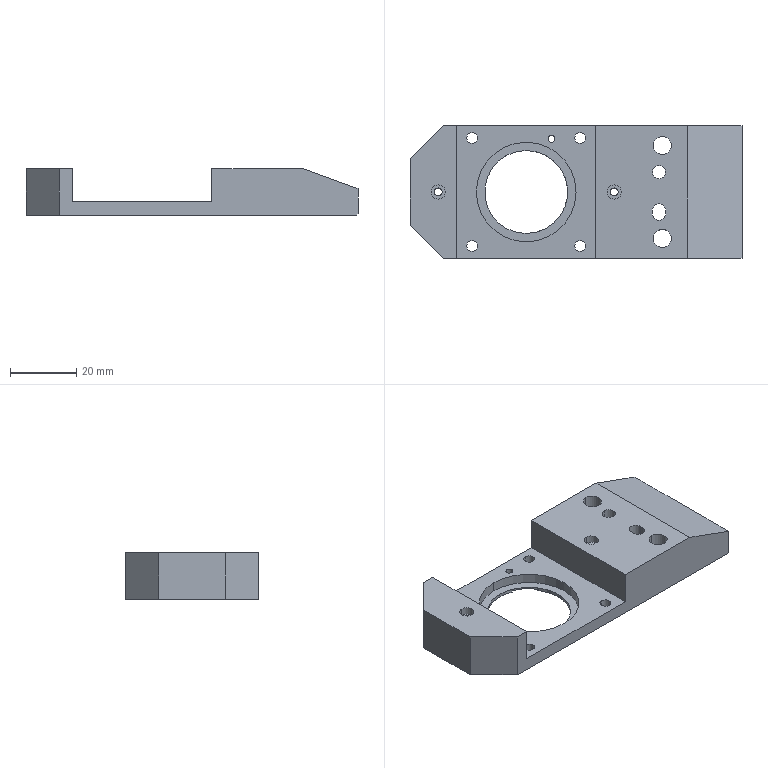NC program | NX | posted with a generic post | part box 100 x 40 x 14 mm
Lines 7056 to 8468 of 15435:
(DRILLING_COPY_1 , TOOL : ZXZ)
N14098 T20 M6
N14100 G54
N14102 G17 G0 G90 X-31.263 Y-16.263 S5000 M3
N14104 G43 Z30. H20
N14106 G94 G81 G98 Z-11. F250. R-7.
N14108 X-41.5 Y0. Z-1. R3.
N14110 X-31.263 Y16.263 Z-11. R-7.
N14112 X-7.4 Y16.
N14114 X1.263 Y16.263
N14116 X-15. Y0.
N14118 X1.263 Y-16.263
N14120 X11.5 Y0. Z-1. R3.
N14122 X26. Y14.
N14124 X25. Y6.
N14126 Y-5.5
N14128 X26. Y-14.
N14130 G80
N14132 G0 X26. Y-14. Z30.
N14134 M5
(DRILLING_COPY_1_COPY , TOOL : 3.3ZT)
N14136 T13 M6
N14138 G54
N14140 G17 G0 G90 X1.263 Y-16.263 S2000 M3
N14142 G43 Z30. H13
N14144 G94 G83 G98 Z-15.491 F150. Q2. R-7.
N14146 X-31.263
N14148 Y16.263
N14150 X1.263
N14152 G80
N14154 G0 X1.263 Y16.263 Z30.
N14156 M5
(TOOLCOMP11 , TOOL : D2.9XYD)
N14158 T11 M6
N14160 G54
N14162 G17 G0 G90 X-31.263 Y16.263 S4000 M3
N14164 G43 Z30. H11
N14166 Z-9.373
N14168 G42 G94 G1 X-31.19 Y16.195 F1000. D11
N14170 G2 X-31.327 Y15.983 Z-9.5 R0.134
N14172 X-31.327 Y15.983 Z-10.2 I0.064 J0.28
N14174 X-31.327 Y15.983 Z-10.9 I0.064 J0.28
N14176 X-31.327 Y15.983 Z-11.6 I0.064 J0.28
N14178 X-31.327 Y15.983 Z-12.3 I0.064 J0.28
N14180 X-31.327 Y15.983 Z-13. I0.064 J0.28
N14182 X-31.327 Y15.983 Z-13.7 I0.064 J0.28
N14184 X-31.327 Y16.544 Z-14. R0.287
N14186 X-31.19 Y16.332 Z-14.127 R0.134
N14188 G40
N14190 G1 X-31.263 Y16.263
N14192 G0 Z30.
N14194 Z-9.359
N14196 G42 G1 X-31.18 Y16.208
N14198 G2 X-31.347 Y15.898 Z-9.5 R0.183
N14200 X-31.347 Y15.898 Z-10.2 I0.083 J0.366
N14202 X-31.347 Y15.898 Z-10.9 I0.083 J0.366
N14204 X-31.347 Y15.898 Z-11.6 I0.083 J0.366
N14206 X-31.347 Y15.898 Z-12.3 I0.083 J0.366
N14208 X-31.347 Y15.898 Z-13. I0.083 J0.366
N14210 X-31.347 Y15.898 Z-13.7 I0.083 J0.366
N14212 X-31.347 Y16.629 Z-14. R0.375
N14214 X-31.18 Y16.319 Z-14.141 R0.183
N14216 G40
N14218 G1 X-31.263 Y16.263
N14220 G0 Z30.
N14222 Z-9.351
N14224 G42 G1 X-31.175 Y16.217
N14226 G2 X-31.366 Y15.813 Z-9.5 R0.229
N14228 X-31.366 Y15.813 Z-10.2 I0.103 J0.451
N14230 X-31.366 Y15.813 Z-10.9 I0.103 J0.451
N14232 X-31.366 Y15.813 Z-11.6 I0.103 J0.451
N14234 X-31.366 Y15.813 Z-12.3 I0.103 J0.451
N14236 X-31.366 Y15.813 Z-13. I0.103 J0.451
N14238 X-31.366 Y15.813 Z-13.7 I0.103 J0.451
N14240 X-31.366 Y16.714 Z-14. R0.462
N14242 X-31.175 Y16.31 Z-14.149 R0.229
N14244 G40
N14246 G1 X-31.263 Y16.263
N14248 G0 Z30.
N14250 Z-9.346
N14252 G42 G1 X-31.172 Y16.223
N14254 G2 X-31.386 Y15.727 Z-9.5 R0.275
N14256 X-31.386 Y15.727 Z-10.2 I0.122 J0.536
N14258 X-31.386 Y15.727 Z-10.9 I0.122 J0.536
N14260 X-31.386 Y15.727 Z-11.6 I0.122 J0.536
N14262 X-31.386 Y15.727 Z-12.3 I0.122 J0.536
N14264 X-31.386 Y15.727 Z-13. I0.122 J0.536
N14266 X-31.386 Y15.727 Z-13.7 I0.122 J0.536
N14268 X-31.386 Y16.8 Z-14. R0.55
N14270 X-31.172 Y16.304 Z-14.154 R0.275
N14272 G40
N14274 G1 X-31.263 Y16.263
N14276 G0 Z30.
N14278 X1.263
N14280 Z-9.373
N14282 G42 G1 X1.337 Y16.195
N14284 G2 X1.199 Y15.983 Z-9.5 R0.134
N14286 X1.199 Y15.983 Z-10.2 I0.064 J0.28
N14288 X1.199 Y15.983 Z-10.9 I0.064 J0.28
N14290 X1.199 Y15.983 Z-11.6 I0.064 J0.28
N14292 X1.199 Y15.983 Z-12.3 I0.064 J0.28
N14294 X1.199 Y15.983 Z-13. I0.064 J0.28
N14296 X1.199 Y15.983 Z-13.7 I0.064 J0.28
N14298 X1.199 Y16.544 Z-14. R0.287
N14300 X1.337 Y16.332 Z-14.127 R0.134
N14302 G40
N14304 G1 X1.263 Y16.263
N14306 G0 Z30.
N14308 Z-9.359
N14310 G42 G1 X1.347 Y16.208
N14312 G2 X1.18 Y15.898 Z-9.5 R0.183
N14314 X1.18 Y15.898 Z-10.2 I0.083 J0.366
N14316 X1.18 Y15.898 Z-10.9 I0.083 J0.366
N14318 X1.18 Y15.898 Z-11.6 I0.083 J0.366
N14320 X1.18 Y15.898 Z-12.3 I0.083 J0.366
N14322 X1.18 Y15.898 Z-13. I0.083 J0.366
N14324 X1.18 Y15.898 Z-13.7 I0.083 J0.366
N14326 X1.18 Y16.629 Z-14. R0.375
N14328 X1.347 Y16.319 Z-14.141 R0.183
N14330 G40
N14332 G1 X1.263 Y16.263
N14334 G0 Z30.
N14336 Z-9.351
N14338 G42 G1 X1.352 Y16.217
N14340 G2 X1.161 Y15.813 Z-9.5 R0.229
N14342 X1.161 Y15.813 Z-10.2 I0.103 J0.451
N14344 X1.161 Y15.813 Z-10.9 I0.103 J0.451
N14346 X1.161 Y15.813 Z-11.6 I0.103 J0.451
N14348 X1.161 Y15.813 Z-12.3 I0.103 J0.451
N14350 X1.161 Y15.813 Z-13. I0.103 J0.451
N14352 X1.161 Y15.813 Z-13.7 I0.103 J0.451
N14354 X1.161 Y16.714 Z-14. R0.462
N14356 X1.352 Y16.31 Z-14.149 R0.229
N14358 G40
N14360 G1 X1.263 Y16.263
N14362 G0 Z30.
N14364 Z-9.346
N14366 G42 G1 X1.355 Y16.223
N14368 G2 X1.141 Y15.727 Z-9.5 R0.275
N14370 X1.141 Y15.727 Z-10.2 I0.122 J0.536
N14372 X1.141 Y15.727 Z-10.9 I0.122 J0.536
N14374 X1.141 Y15.727 Z-11.6 I0.122 J0.536
N14376 X1.141 Y15.727 Z-12.3 I0.122 J0.536
N14378 X1.141 Y15.727 Z-13. I0.122 J0.536
N14380 X1.141 Y15.727 Z-13.7 I0.122 J0.536
N14382 X1.141 Y16.8 Z-14. R0.55
N14384 X1.355 Y16.304 Z-14.154 R0.275
N14386 G40
N14388 G1 X1.263 Y16.263
N14390 G0 Z30.
N14392 X-31.263 Y-16.263
N14394 Z-9.373
N14396 G42 G1 X-31.19 Y-16.332
N14398 G2 X-31.327 Y-16.544 Z-9.5 R0.134
N14400 X-31.327 Y-16.544 Z-10.2 I0.064 J0.28
N14402 X-31.327 Y-16.544 Z-10.9 I0.064 J0.28
N14404 X-31.327 Y-16.544 Z-11.6 I0.064 J0.28
N14406 X-31.327 Y-16.544 Z-12.3 I0.064 J0.28
N14408 X-31.327 Y-16.544 Z-13. I0.064 J0.28
N14410 X-31.327 Y-16.544 Z-13.7 I0.064 J0.28
N14412 X-31.327 Y-15.983 Z-14. R0.287
N14414 X-31.19 Y-16.195 Z-14.127 R0.134
N14416 G40
N14418 G1 X-31.263 Y-16.263
N14420 G0 Z30.
N14422 Z-9.359
N14424 G42 G1 X-31.18 Y-16.319
N14426 G2 X-31.347 Y-16.629 Z-9.5 R0.183
N14428 X-31.347 Y-16.629 Z-10.2 I0.083 J0.366
N14430 X-31.347 Y-16.629 Z-10.9 I0.083 J0.366
N14432 X-31.347 Y-16.629 Z-11.6 I0.083 J0.366
N14434 X-31.347 Y-16.629 Z-12.3 I0.083 J0.366
N14436 X-31.347 Y-16.629 Z-13. I0.083 J0.366
N14438 X-31.347 Y-16.629 Z-13.7 I0.083 J0.366
N14440 X-31.347 Y-15.898 Z-14. R0.375
N14442 X-31.18 Y-16.208 Z-14.141 R0.183
N14444 G40
N14446 G1 X-31.263 Y-16.263
N14448 G0 Z30.
N14450 Z-9.351
N14452 G42 G1 X-31.175 Y-16.31
N14454 G2 X-31.366 Y-16.714 Z-9.5 R0.229
N14456 X-31.366 Y-16.714 Z-10.2 I0.103 J0.451
N14458 X-31.366 Y-16.714 Z-10.9 I0.103 J0.451
N14460 X-31.366 Y-16.714 Z-11.6 I0.103 J0.451
N14462 X-31.366 Y-16.714 Z-12.3 I0.103 J0.451
N14464 X-31.366 Y-16.714 Z-13. I0.103 J0.451
N14466 X-31.366 Y-16.714 Z-13.7 I0.103 J0.451
N14468 X-31.366 Y-15.813 Z-14. R0.462
N14470 X-31.175 Y-16.217 Z-14.149 R0.229
N14472 G40
N14474 G1 X-31.263 Y-16.263
N14476 G0 Z30.
N14478 Z-9.346
N14480 G42 G1 X-31.172 Y-16.304
N14482 G2 X-31.386 Y-16.8 Z-9.5 R0.275
N14484 X-31.386 Y-16.8 Z-10.2 I0.122 J0.536
N14486 X-31.386 Y-16.8 Z-10.9 I0.122 J0.536
N14488 X-31.386 Y-16.8 Z-11.6 I0.122 J0.536
N14490 X-31.386 Y-16.8 Z-12.3 I0.122 J0.536
N14492 X-31.386 Y-16.8 Z-13. I0.122 J0.536
N14494 X-31.386 Y-16.8 Z-13.7 I0.122 J0.536
N14496 X-31.386 Y-15.727 Z-14. R0.55
N14498 X-31.172 Y-16.223 Z-14.154 R0.275
N14500 G40
N14502 G1 X-31.263 Y-16.263
N14504 G0 Z30.
N14506 X1.263
N14508 Z-9.373
N14510 G42 G1 X1.337 Y-16.332
N14512 G2 X1.199 Y-16.544 Z-9.5 R0.134
N14514 X1.199 Y-16.544 Z-10.2 I0.064 J0.28
N14516 X1.199 Y-16.544 Z-10.9 I0.064 J0.28
N14518 X1.199 Y-16.544 Z-11.6 I0.064 J0.28
N14520 X1.199 Y-16.544 Z-12.3 I0.064 J0.28
N14522 X1.199 Y-16.544 Z-13. I0.064 J0.28
N14524 X1.199 Y-16.544 Z-13.7 I0.064 J0.28
N14526 X1.199 Y-15.983 Z-14. R0.287
N14528 X1.337 Y-16.195 Z-14.127 R0.134
N14530 G40
N14532 G1 X1.263 Y-16.263
N14534 G0 Z30.
N14536 Z-9.359
N14538 G42 G1 X1.347 Y-16.319
N14540 G2 X1.18 Y-16.629 Z-9.5 R0.183
N14542 X1.18 Y-16.629 Z-10.2 I0.083 J0.366
N14544 X1.18 Y-16.629 Z-10.9 I0.083 J0.366
N14546 X1.18 Y-16.629 Z-11.6 I0.083 J0.366
N14548 X1.18 Y-16.629 Z-12.3 I0.083 J0.366
N14550 X1.18 Y-16.629 Z-13. I0.083 J0.366
N14552 X1.18 Y-16.629 Z-13.7 I0.083 J0.366
N14554 X1.18 Y-15.898 Z-14. R0.375
N14556 X1.347 Y-16.208 Z-14.141 R0.183
N14558 G40
N14560 G1 X1.263 Y-16.263
N14562 G0 Z30.
N14564 Z-9.351
N14566 G42 G1 X1.352 Y-16.31
N14568 G2 X1.161 Y-16.714 Z-9.5 R0.229
N14570 X1.161 Y-16.714 Z-10.2 I0.103 J0.451
N14572 X1.161 Y-16.714 Z-10.9 I0.103 J0.451
N14574 X1.161 Y-16.714 Z-11.6 I0.103 J0.451
N14576 X1.161 Y-16.714 Z-12.3 I0.103 J0.451
N14578 X1.161 Y-16.714 Z-13. I0.103 J0.451
N14580 X1.161 Y-16.714 Z-13.7 I0.103 J0.451
N14582 X1.161 Y-15.813 Z-14. R0.462
N14584 X1.352 Y-16.217 Z-14.149 R0.229
N14586 G40
N14588 G1 X1.263 Y-16.263
N14590 G0 Z30.
N14592 Z-9.346
N14594 G42 G1 X1.355 Y-16.304
N14596 G2 X1.141 Y-16.8 Z-9.5 R0.275
N14598 X1.141 Y-16.8 Z-10.2 I0.122 J0.536
N14600 X1.141 Y-16.8 Z-10.9 I0.122 J0.536
N14602 X1.141 Y-16.8 Z-11.6 I0.122 J0.536
N14604 X1.141 Y-16.8 Z-12.3 I0.122 J0.536
N14606 X1.141 Y-16.8 Z-13. I0.122 J0.536
N14608 X1.141 Y-16.8 Z-13.7 I0.122 J0.536
N14610 X1.141 Y-15.727 Z-14. R0.55
N14612 X1.355 Y-16.223 Z-14.154 R0.275
N14614 G40
N14616 G1 X1.263 Y-16.263
N14618 G0 Z30.
N14620 M5
(DRILLING_COPY_1_COPY_COPY_2 , TOOL : 2.1ZT)
N14622 T15 M6
N14624 G54
N14626 G17 G0 G90 X-7.4 Y16. S2001 M3
N14628 G43 Z30. H15
N14630 G94 G83 G98 Z-14.616 F120. Q2. R-7.
N14632 G80
N14634 G0 X-7.4 Y16. Z30.
N14636 M5
(TOOLCOMP7 , TOOL : 1.95XYD)
N14638 T07 M6
N14640 G54
N14642 G17 G0 G90 X-7.4 Y16. S4000 M3
N14644 G43 Z30. H7
N14646 Z-9.475
N14648 G42 G94 G1 X-7.343 Y16.082 F1000. D7
N14650 X-7.333 Y16.099 Z-9.483
N14652 X-7.313 Y16.098 Z-9.492
N14654 X-7.304 Y16.08 Z-9.5
N14656 G2 X-7.304 Y16.08 Z-9.95 I-0.096 J-0.08
N14658 X-7.304 Y16.08 Z-10.4 I-0.096 J-0.08
N14660 X-7.304 Y16.08 Z-10.85 I-0.096 J-0.08
N14662 X-7.304 Y16.08 Z-11.3 I-0.096 J-0.08
N14664 X-7.304 Y16.08 Z-11.75 I-0.096 J-0.08
N14666 X-7.304 Y16.08 Z-12.2 I-0.096 J-0.08
N14668 X-7.304 Y16.08 Z-12.65 I-0.096 J-0.08
N14670 X-7.304 Y16.08 Z-13.1 I-0.096 J-0.08
N14672 X-7.378 Y16.123 Z-13.5 R-0.125
N14674 G1 X-7.359 Y16.124 Z-13.508
N14676 X-7.348 Y16.108 Z-13.517
N14678 X-7.358 Y16.091 Z-13.525
N14680 G40
N14682 X-7.4 Y16.
N14684 G0 Z30.
N14686 Z-9.437
N14688 G42 G1 X-7.388 Y16.099
N14690 X-7.359 Y16.154 Z-9.458
N14692 X-7.295 Y16.167 Z-9.479
N14694 X-7.247 Y16.129 Z-9.5
N14696 G2 X-7.247 Y16.129 Z-9.95 I-0.153 J-0.129
N14698 X-7.247 Y16.129 Z-10.4 I-0.153 J-0.129
N14700 X-7.247 Y16.129 Z-10.85 I-0.153 J-0.129
N14702 X-7.247 Y16.129 Z-11.3 I-0.153 J-0.129
N14704 X-7.247 Y16.129 Z-11.75 I-0.153 J-0.129
N14706 X-7.247 Y16.129 Z-12.2 I-0.153 J-0.129
N14708 X-7.247 Y16.129 Z-12.65 I-0.153 J-0.129
N14710 X-7.247 Y16.129 Z-13.1 I-0.153 J-0.129
N14712 X-7.365 Y16.197 Z-13.5 R-0.2
N14714 G1 X-7.308 Y16.174 Z-13.521
N14716 X-7.287 Y16.113 Z-13.542
N14718 X-7.32 Y16.06 Z-13.563
N14720 G40
N14722 X-7.4 Y16.
N14724 G0 Z30.
N14726 Z-9.42
N14728 G42 G1 X-7.414 Y16.099
N14730 G2 X-7.189 Y16.177 Z-9.5 R0.127
N14732 X-7.189 Y16.177 Z-9.95 I-0.211 J-0.177
N14734 X-7.189 Y16.177 Z-10.4 I-0.211 J-0.177
N14736 X-7.189 Y16.177 Z-10.85 I-0.211 J-0.177
N14738 X-7.189 Y16.177 Z-11.3 I-0.211 J-0.177
N14740 X-7.189 Y16.177 Z-11.75 I-0.211 J-0.177
N14742 X-7.189 Y16.177 Z-12.2 I-0.211 J-0.177
N14744 X-7.189 Y16.177 Z-12.65 I-0.211 J-0.177
N14746 X-7.189 Y16.177 Z-13.1 I-0.211 J-0.177
N14748 X-7.352 Y16.271 Z-13.5 R-0.275
N14750 X-7.307 Y16.037 Z-13.58 R0.127
N14752 G40
N14754 G1 X-7.4 Y16.
N14756 G0 Z30.
N14758 M5
(DRILLING_COPY_2 , TOOL : 3.8ZT)
N14760 T09 M6
N14762 G54
N14764 G17 G0 G90 X25. Y6. S2000 M3
N14766 G43 Z11. H9
N14768 G94 G83 G98 Z-15.642 F150. Q2. R3.
N14770 Y-5.5 Z-15.202
N14772 G80
N14774 M5
(DRILLING_COPY_2_COPY , TOOL : 4.0JD)
N14776 T10 M6
N14778 G54
N14780 G17 G0 G90 X25. Y6. S1000 M3
N14782 G43 Z11. H10
N14784 G94 G85 G98 Z-14.5 F50. R3.
N14786 G80
N14788 M5
(DRILLING_COPY_1_COPY_COPY , TOOL : 5.5ZT)
N14790 T12 M6
N14792 G54
N14794 G17 G0 G90 X26. Y-14. S1215 M3
N14796 G43 Z30. H12
N14798 G94 G83 G98 Z-15.652 F150. Q2. R3.
N14800 Y14.
N14802 G80
N14804 G0 X26. Y14. Z30.
N14806 M5
(DRILLING_COPY_1_COPY_COPY_1 , TOOL : 2.4ZT)
N14808 T19 M6
N14810 G54
N14812 G17 G0 G90 X-41.5 Y0. S2785 M3
N14814 G43 Z30. H19
N14816 G94 G83 G98 Z-14.721 F100. Q2. R3.
N14818 X11.5
N14820 G80
N14822 G0 X11.5 Y0. Z30.
N14824 M5
(ZLEVEL_PROFILE_1_COPY , TOOL : D10JING)
N14826 T14 M6
N14828 G54
N14830 G17 G0 G90 X-16.222 Y-6.384 S6500 M3
N14832 G43 Z30. H14
N14834 Z-13.
N14836 G94 G1 Z-14. F1000.
N14838 X-15.866 Y-7.
N14840 G3 X-15. Y-7.5 R1.
N14842 X-7.5 Y0. R7.5
N14844 X-15. Y-7.5 R-7.5
N14846 X-14.134 Y-7. R1.
N14848 G1 X-13.778 Y-6.384
N14850 Z-13.
N14852 G0 Z53.
N14854 X51.096 Y-25.899
N14856 Z-13.
N14858 G1 Z-14.
N14860 X50.866 Y-25.5
N14862 G3 X50. Y-25. R1.
N14864 G1 X-40.
N14866 G2 X-43.536 Y-23.536 R5.
N14868 G1 X-53.536 Y-13.536
N14870 G2 X-55. Y-10. R5.
N14872 G1 Y10.
N14874 G2 X-53.536 Y13.536 R5.
N14876 G1 X-43.536 Y23.536
N14878 G2 X-40. Y25. R5.
N14880 G1 X50.
N14882 G2 X55. Y20. R5.
N14884 G1 Y-20.
N14886 G2 X50. Y-25. R5.
N14888 G3 X49.134 Y-25.5 R1.
N14890 G1 X48.845 Y-26.
N14892 Z-13.
N14894 G0 Z30.
(FLOOR_WALL , TOOL : D10JING)
N14896 X-29.999
N14898 Z-9.
N14900 G1 Z-10. F1250.
N14902 Y-24.134
N14904 G3 X-30.499 Y-25. R1.
N14906 G1 Y25.
N14908 X-26.071
N14910 Y-25.
N14912 X-21.642
N14914 Y25.
N14916 X-17.214
N14918 Y-25.
N14920 X-12.785
N14922 Y25.
N14924 X-8.357
N14926 Y-25.
N14928 X-3.928
N14930 Y25.
N14932 X0.5
N14934 Y-25.
N14936 G2 X0. Y-25.866 R1.
N14938 G1 X-0.232 Y-26.
N14940 Z-9.
N14942 G0 Z30.
N14944 X0.268
N14946 Z-9.
N14948 G1 Z-10.
N14950 X0.5 Y-25.866
N14952 G3 X1. Y-25. R1.
N14954 G1 Y25.
N14956 G3 X0.5 Y25.866 R1.
N14958 G1 X0.268 Y26.
N14960 Z-9.
N14962 G0 Z30.
N14964 X-30.268
N14966 Z-9.
N14968 G1 Z-10.
N14970 X-30.5 Y25.866
N14972 G3 X-31. Y25. R1.
N14974 G1 Y-25.
N14976 G3 X-30.5 Y-25.866 R1.
N14978 G1 X-30.268 Y-26.
N14980 Z-9.
N14982 G0 Z30.
N14984 M5
(ZLEVEL_PROFILE_COPY_COPY_COPY_COPY , TOOL : D6R0.5)
N14986 T08 M6
N14988 G54
N14990 G17 G0 G90 X37.281 Y22.451 S6500 M3
N14992 G43 Z30. H8
N14994 Z0.966
N14996 G94 G1 Z-0.034 F1000.
N14998 X36.496 Y21.997
N15000 G3 X36.196 Y21.477 R0.6
N15002 G1 X36.197 Y20. F2500.
N15004 Y-20.
N15006 X36.196 Y-21.477
N15008 X36.244 Z-0.051
N15010 X36.29 Y-21.478 Z-0.068
N15012 X36.291 Y-20.
N15014 Y20.
N15016 X36.29 Y21.478
N15018 X36.338 Z-0.086
N15020 X36.384 Z-0.103
N15022 X36.385 Y20.
N15024 Y-20.
N15026 X36.384 Y-21.478
N15028 X36.432 Y-21.479 Z-0.12
N15030 X36.478 Z-0.137
N15032 X36.479 Y-20.
N15034 Y20.
N15036 X36.478 Y21.479
N15038 X36.526 Z-0.154
N15040 X36.572 Z-0.171
N15042 X36.573 Y20.
N15044 Y-20.
N15046 X36.572 Y-21.479
N15048 X36.62 Y-21.48 Z-0.188
N15050 X36.666 Z-0.205
N15052 X36.667 Y-20.
N15054 Y20.
N15056 X36.666 Y21.48
N15058 X36.714 Z-0.222
N15060 X36.76 Z-0.239
N15062 X36.761 Y20.
N15064 Y-20.
N15066 X36.76 Y-21.48
N15068 X36.808 Y-21.481 Z-0.257
N15070 X36.854 Z-0.274
N15072 X36.855 Y-20.
N15074 Y20.
N15076 X36.854 Y21.481
N15078 X36.902 Z-0.291
N15080 X36.948 Y21.482 Z-0.308
N15082 X36.949 Y20.
N15084 Y-20.
N15086 X36.948 Y-21.482
N15088 X36.996 Z-0.325
N15090 X37.042 Z-0.342
N15092 X37.043 Y-20.
N15094 Y20.
N15096 X37.042 Y21.482
N15098 X37.09 Z-0.359
N15100 X37.136 Y21.483 Z-0.376
N15102 X37.137 Y20.
N15104 Y-20.
N15106 X37.136 Y-21.483
N15108 X37.184 Z-0.393
N15110 X37.23 Z-0.41
N15112 X37.231 Y-20.
N15114 Y20.
N15116 X37.23 Y21.483
N15118 X37.278 Z-0.428
N15120 X37.324 Y21.484 Z-0.445
N15122 X37.325 Y20.
N15124 Y-20.
N15126 X37.324 Y-21.484
N15128 X37.372 Z-0.462
N15130 X37.418 Z-0.479
N15132 X37.419 Y-20.
N15134 Y20.
N15136 X37.418 Y21.484
N15138 X37.466 Y21.485 Z-0.496
N15140 X37.512 Z-0.513
N15142 X37.513 Y20.
N15144 Y-20.
N15146 X37.512 Y-21.485
N15148 X37.56 Z-0.53
N15150 X37.606 Z-0.547
N15152 X37.607 Y-20.
N15154 Y20.
N15156 X37.606 Y21.485
N15158 X37.654 Y21.486 Z-0.564
N15160 X37.7 Z-0.581
N15162 X37.701 Y20.
N15164 Y-20.
N15166 X37.7 Y-21.486
N15168 X37.748 Z-0.599
N15170 X37.794 Y-21.487 Z-0.616
N15172 X37.795 Y-20.
N15174 Y20.
N15176 X37.794 Y21.487
N15178 X37.842 Z-0.633
N15180 X37.888 Z-0.65
N15182 X37.889 Y20.
N15184 Y-20.
N15186 X37.888 Y-21.487
N15188 X37.936 Z-0.667
N15190 X37.982 Y-21.488 Z-0.684
N15192 X37.983 Y-20.
N15194 Y20.
N15196 X37.982 Y21.488
N15198 X38.03 Z-0.701
N15200 X38.076 Z-0.718
N15202 X38.077 Y20.
N15204 Y-20.
N15206 X38.076 Y-21.488
N15208 X38.124 Z-0.735
N15210 X38.17 Z-0.752
N15212 X38.171 Y-20.
N15214 Y20.
N15216 X38.17 Y21.489
N15218 X38.218 Z-0.77
N15220 X38.264 Z-0.787
N15222 X38.265 Y20.
N15224 Y-20.
N15226 X38.264 Y-21.489
N15228 X38.312 Z-0.804
N15230 X38.358 Z-0.821
N15232 X38.359 Y-20.
N15234 Y20.
N15236 X38.358 Y21.489
N15238 X38.406 Y21.49 Z-0.838
N15240 X38.452 Z-0.855
N15242 X38.453 Y20.
N15244 Y-20.
N15246 X38.452 Y-21.49
N15248 X38.5 Z-0.872
N15250 X38.546 Z-0.889
N15252 X38.547 Y-20.
N15254 Y20.
N15256 X38.546 Y21.49
N15258 X38.593 Z-0.906
N15260 X38.64 Y21.491 Z-0.923
N15262 Y20.
N15264 Y-20.
N15266 Y-21.491
N15268 X38.687 Z-0.941
N15270 X38.734 Z-0.958
N15272 Y-20.
N15274 Y20.
N15276 Y21.491
N15278 X38.781 Z-0.975
N15280 X38.828 Z-0.992
N15282 Y20.
N15284 Y-20.
N15286 Y-21.491
N15288 X38.875 Y-21.492 Z-1.009
N15290 X38.922 Z-1.026
N15292 Y-20.
N15294 Y20.
N15296 Y21.492
N15298 X38.969 Z-1.043
N15300 X39.016 Z-1.06
N15302 Y20.
N15304 Y-20.
N15306 Y-21.492
N15308 X39.063 Z-1.077
N15310 X39.11 Z-1.094
N15312 Y-20.
N15314 Y20.
N15316 Y21.492
N15318 X39.157 Y21.493 Z-1.112
N15320 X39.204 Z-1.129
N15322 Y20.
N15324 Y-20.
N15326 Y-21.493
N15328 X39.251 Z-1.146
N15330 X39.298 Z-1.163
N15332 Y-20.
N15334 Y20.
N15336 Y21.493
N15338 X39.345 Z-1.18
N15340 X39.392 Z-1.197
N15342 Y20.
N15344 Y-20.
N15346 Y-21.494
N15348 X39.439 Z-1.214
N15350 X39.485 Z-1.231
N15352 X39.486 Y-20.
N15354 Y20.
N15356 X39.485 Y21.494
N15358 X39.533 Z-1.248
N15360 X39.579 Z-1.265
N15362 X39.58 Y20.
N15364 Y-20.
N15366 X39.579 Y-21.494
N15368 X39.627 Z-1.283
N15370 X39.673 Y-21.495 Z-1.3
N15372 X39.674 Y-20.
N15374 Y20.
N15376 X39.673 Y21.495
N15378 X39.721 Z-1.317
N15380 X39.767 Z-1.334
N15382 X39.768 Y20.
N15384 Y-20.
N15386 X39.767 Y-21.495
N15388 X39.815 Z-1.351
N15390 X39.861 Z-1.368
N15392 X39.862 Y-20.
N15394 Y20.
N15396 X39.861 Y21.495
N15398 X39.909 Z-1.385
N15400 X39.955 Z-1.402
N15402 X39.956 Y20.
N15404 Y-20.
N15406 X39.955 Y-21.496
N15408 X40.003 Z-1.419
N15410 X40.049 Z-1.436
N15412 X40.05 Y-20.
N15414 Y20.
N15416 X40.049 Y21.496
N15418 X40.097 Z-1.454
N15420 X40.143 Z-1.471
N15422 X40.144 Y20.
N15424 Y-20.
N15426 X40.143 Y-21.496
N15428 X40.191 Z-1.488
N15430 X40.237 Z-1.505
N15432 X40.238 Y-20.
N15434 Y20.
N15436 X40.237 Y21.496
N15438 X40.285 Z-1.522
N15440 X40.331 Z-1.539
N15442 X40.332 Y20.
N15444 Y-20.
N15446 X40.331 Y-21.496
N15448 X40.379 Z-1.556
N15450 X40.425 Z-1.573
N15452 X40.426 Y-20.
N15454 Y20.
N15456 X40.425 Y21.496
N15458 X40.473 Z-1.59
N15460 X40.519 Y21.497 Z-1.607
N15462 X40.52 Y20.
N15464 Y-20.
N15466 X40.519 Y-21.497
N15468 X40.567 Z-1.625
N15470 X40.613 Z-1.642
N15472 X40.614 Y-20.
N15474 Y20.
N15476 X40.613 Y21.497
N15478 X40.661 Z-1.659
N15480 X40.707 Z-1.676
N15482 X40.708 Y20.
N15484 Y-20.
N15486 X40.707 Y-21.497
N15488 X40.755 Z-1.693
N15490 X40.801 Z-1.71
N15492 X40.802 Y-20.
N15494 Y20.
N15496 X40.801 Y21.497
N15498 X40.849 Z-1.727
N15500 X40.895 Z-1.744
N15502 X40.896 Y20.
N15504 Y-20.
N15506 X40.895 Y-21.497
N15508 X40.943 Z-1.761
N15510 X40.989 Z-1.779
N15512 X40.99 Y-20.
N15514 Y20.
N15516 X40.989 Y21.497
N15518 X41.037 Y21.498 Z-1.796
N15520 X41.083 Z-1.813
N15522 X41.084 Y20.
N15524 Y-20.
N15526 X41.083 Y-21.498
N15528 X41.131 Z-1.83
N15530 X41.177 Z-1.847
N15532 X41.178 Y-20.
N15534 Y20.
N15536 X41.177 Y21.498
N15538 X41.225 Z-1.864
N15540 X41.271 Z-1.881
N15542 X41.272 Y20.
N15544 Y-20.
N15546 X41.271 Y-21.498
N15548 X41.319 Z-1.898
N15550 X41.365 Z-1.915
N15552 X41.366 Y-20.
N15554 Y20.
N15556 X41.365 Y21.498
N15558 X41.413 Z-1.932
N15560 X41.459 Z-1.95
N15562 X41.46 Y20.
N15564 Y-20.
N15566 X41.459 Y-21.498
N15568 X41.507 Z-1.967
N15570 X41.553 Z-1.984
N15572 X41.554 Y-20.
N15574 Y20.
N15576 X41.553 Y21.499
N15578 X41.601 Z-2.001
N15580 X41.647 Z-2.018
N15582 Y20.
N15584 Y-20.
N15586 Y-21.498
N15588 X41.694 Y-21.499 Z-2.035
N15590 X41.741 Z-2.052
N15592 Y-20.
N15594 Y20.
N15596 Y21.499
N15598 X41.788 Z-2.069
N15600 X41.835 Z-2.086
N15602 Y20.
N15604 Y-20.
N15606 Y-21.499
N15608 X41.882 Z-2.103
N15610 X41.929 Z-2.121
N15612 Y-20.
N15614 Y20.
N15616 Y21.499
N15618 X41.976 Z-2.138
N15620 X42.023 Z-2.155
N15622 Y20.
N15624 Y-20.
N15626 Y-21.499
N15628 X42.07 Z-2.172
N15630 X42.117 Z-2.189
N15632 Y-20.
N15634 Y20.
N15636 Y21.499
N15638 X42.164 Z-2.206
N15640 X42.211 Z-2.223
N15642 Y20.
N15644 Y-20.
N15646 Y-21.499
N15648 X42.258 Z-2.24
N15650 X42.305 Z-2.257
N15652 Y-20.
N15654 Y20.
N15656 Y21.499
N15658 X42.352 Z-2.274
N15660 X42.399 Z-2.292
N15662 Y20.
N15664 Y-20.
N15666 Y-21.499
N15668 X42.446 Z-2.309
N15670 X42.493 Z-2.326
N15672 Y-20.
N15674 Y20.
N15676 Y21.499
N15678 X42.54 Z-2.343
N15680 X42.587 Z-2.36
N15682 Y20.
N15684 Y-20.
N15686 Y-21.499
N15688 X42.634 Z-2.377
N15690 X42.681 Z-2.394
N15692 Y-20.
N15694 Y20.
N15696 Y21.499
N15698 X42.728 Z-2.411
N15700 X42.775 Z-2.428
N15702 Y20.
N15704 Y-20.
N15706 Y-21.499
N15708 X42.822 Z-2.445
N15710 X42.868 Z-2.463
N15712 X42.869 Y-20.
N15714 Y20.
N15716 X42.868 Y21.499
N15718 X42.916 Z-2.48
N15720 X42.963 Z-2.497
N15722 Y20.
N15724 Y-20.
N15726 Y-21.499
N15728 X43.01 Z-2.514
N15730 X43.056 Z-2.531
N15732 X43.057 Y-20.
N15734 Y20.
N15736 X43.056 Y21.499
N15738 X43.104 Z-2.548
N15740 X43.15 Z-2.565
N15742 X43.151 Y20.
N15744 Y-20.
N15746 X43.15 Y-21.499
N15748 X43.198 Z-2.582
N15750 X43.244 Z-2.599
N15752 X43.245 Y-20.
N15754 Y20.
N15756 X43.244 Y21.5
N15758 X43.292 Z-2.616
N15760 X43.338 Z-2.634
N15762 X43.339 Y20.
N15764 Y-20.
N15766 X43.338 Y-21.499
N15768 X43.386 Z-2.651
N15770 X43.432 Y-21.5 Z-2.668
N15772 X43.433 Y-20.
N15774 Y20.
N15776 X43.432 Y21.5
N15778 X43.48 Z-2.685
N15780 X43.526 Z-2.702
N15782 X43.527 Y20.
N15784 Y-20.
N15786 X43.526 Y-21.5
N15788 X43.574 Z-2.719
N15790 X43.62 Z-2.736
N15792 X43.621 Y-20.
N15794 Y20.
N15796 X43.62 Y21.5
N15798 X43.668 Z-2.753
N15800 X43.714 Z-2.77
N15802 X43.715 Y20.
N15804 Y-20.
N15806 X43.714 Y-21.5
N15808 X43.762 Z-2.787
N15810 X43.808 Z-2.805
N15812 X43.809 Y-20.
N15814 Y20.
N15816 X43.808 Y21.5
N15818 X43.856 Z-2.822
N15820 X43.902 Z-2.839
N15822 X43.903 Y20.
N15824 Y-20.
N15826 X43.902 Y-21.5
N15828 X43.95 Z-2.856
N15830 X43.996 Z-2.873
N15832 X43.997 Y-20.
N15834 Y20.
N15836 X43.996 Y21.5
N15838 X44.044 Z-2.89
N15840 X44.09 Z-2.907
N15842 X44.091 Y20.
N15844 Y-20.
N15846 X44.09 Y-21.5
N15848 X44.138 Z-2.924
N15850 X44.184 Z-2.941
N15852 X44.185 Y-20.
N15854 Y20.
N15856 X44.184 Y21.5
N15858 X44.232 Z-2.958
N15860 X44.278 Z-2.976
N15862 X44.279 Y20.
N15864 Y-20.
N15866 X44.278 Y-21.5
N15868 X44.326 Z-2.993
N15870 X44.372 Z-3.01
N15872 X44.373 Y-20.
N15874 Y20.
N15876 X44.372 Y21.5
N15878 X44.42 Z-3.027
N15880 X44.466 Z-3.044
N15882 X44.467 Y20.
N15884 Y-20.
N15886 X44.466 Y-21.5
N15888 X44.514 Z-3.061
N15890 X44.56 Z-3.078
N15892 X44.561 Y-20.
N15894 Y20.
N15896 X44.56 Y21.5
N15898 X44.608 Z-3.095
N15900 X44.654 Z-3.112
N15902 X44.655 Y20.
N15904 Y-20.
N15906 X44.654 Y-21.5
N15908 X44.701 Z-3.129
N15910 X44.748 Z-3.147
N15912 Y-20.
N15914 Y20.
N15916 Y21.5
N15918 X44.795 Z-3.164
N15920 X44.842 Z-3.181
N15922 Y20.
N15924 Y-20.
N15926 Y-21.5
N15928 X44.889 Z-3.198
N15930 X44.936 Z-3.215
N15932 Y-20.
N15934 Y20.
N15936 Y21.5
N15938 X44.983 Z-3.232
N15940 X45.03 Z-3.249
N15942 Y20.
N15944 Y-20.
N15946 Y-21.5
N15948 X45.077 Z-3.266
N15950 X45.124 Z-3.283
N15952 Y-20.
N15954 Y20.
N15956 Y21.5
N15958 X45.171 Z-3.3
N15960 X45.218 Z-3.318
N15962 Y20.
N15964 Y-20.
N15966 Y-21.5
N15968 X45.265 Z-3.335
N15970 X45.312 Z-3.352
N15972 Y-20.
N15974 Y20.
N15976 Y21.5
N15978 X45.359 Z-3.369
N15980 X45.406 Z-3.386
N15982 Y20.
N15984 Y-20.
N15986 Y-21.5
N15988 X45.453 Z-3.403
N15990 X45.5 Z-3.42
N15992 Y-20.
N15994 Y20.
N15996 Y21.5
N15998 X45.547 Z-3.437
N16000 X45.594 Y21.499 Z-3.454
N16002 Y20.
N16004 Y-20.
N16006 Y-21.5
N16008 X45.641 Y-21.499 Z-3.472
N16010 X45.688 Z-3.489
N16012 Y-20.
N16014 Y20.
N16016 Y21.499
N16018 X45.735 Z-3.506
N16020 X45.782 Z-3.523
N16022 Y20.
N16024 Y-20.
N16026 Y-21.499
N16028 X45.829 Z-3.54
N16030 X45.875 Z-3.557
N16032 X45.876 Y-20.
N16034 Y20.
N16036 X45.875 Y21.499
N16038 X45.923 Z-3.574
N16040 X45.969 Z-3.591
N16042 X45.97 Y20.
N16044 Y-20.
N16046 X45.969 Y-21.499
N16048 X46.017 Z-3.608
N16050 X46.063 Z-3.625
N16052 X46.064 Y-20.
N16054 Y20.
N16056 X46.063 Y21.499
N16058 X46.111 Z-3.643
N16060 X46.157 Z-3.66
N16062 X46.158 Y20.
N16064 Y-20.
N16066 X46.157 Y-21.499
N16068 X46.205 Z-3.677
N16070 X46.251 Z-3.694
N16072 X46.252 Y-20.
N16074 Y20.
N16076 X46.251 Y21.499
N16078 X46.299 Z-3.711
N16080 X46.345 Z-3.728
N16082 X46.346 Y20.
N16084 Y-20.
N16086 X46.345 Y-21.499
N16088 X46.393 Z-3.745
N16090 X46.439 Z-3.762
N16092 X46.44 Y-20.
N16094 Y20.
N16096 X46.439 Y21.499
N16098 X46.487 Z-3.779
N16100 X46.533 Z-3.796
N16102 X46.534 Y20.
N16104 Y-20.
N16106 X46.533 Y-21.499
N16108 X46.581 Z-3.814
N16110 X46.627 Z-3.831
N16112 X46.628 Y-20.
N16114 Y20.
N16116 X46.627 Y21.499
N16118 X46.675 Z-3.848
N16120 X46.721 Z-3.865
N16122 X46.722 Y20.
N16124 Y-20.
N16126 X46.721 Y-21.499
N16128 X46.769 Z-3.882
N16130 X46.815 Z-3.899
N16132 X46.816 Y-20.
N16134 Y20.
N16136 X46.815 Y21.499
N16138 X46.863 Z-3.916
N16140 X46.909 Z-3.933
N16142 X46.91 Y20.
N16144 Y-20.
N16146 X46.909 Y-21.499
N16148 X46.957 Z-3.95
N16150 X47.003 Z-3.967
N16152 X47.004 Y-20.
N16154 Y20.
N16156 X47.003 Y21.499
N16158 X47.051 Z-3.985
N16160 X47.097 Z-4.002
N16162 X47.098 Y20.
N16164 Y-20.
N16166 X47.097 Y-21.499
N16168 X47.145 Z-4.019
N16170 X47.191 Z-4.036
N16172 X47.192 Y-20.
N16174 Y20.
N16176 X47.191 Y21.499
N16178 X47.239 Y21.498 Z-4.053
N16180 X47.285 Z-4.07
N16182 X47.286 Y20.
N16184 Y-20.
N16186 X47.285 Y-21.498
N16188 X47.333 Z-4.087
N16190 X47.379 Z-4.104
N16192 X47.38 Y-20.
N16194 Y20.
N16196 X47.379 Y21.498
N16198 X47.427 Z-4.121
N16200 X47.473 Z-4.138
N16202 X47.474 Y20.
N16204 Y-20.
N16206 X47.473 Y-21.498
N16208 X47.521 Z-4.156
N16210 X47.567 Z-4.173
N16212 X47.568 Y-20.
N16214 Y20.
N16216 X47.567 Y21.498
N16218 X47.615 Z-4.19
N16220 X47.661 Z-4.207
N16222 X47.662 Y20.
N16224 Y-20.
N16226 X47.661 Y-21.498
N16228 X47.709 Z-4.224
N16230 X47.755 Z-4.241
N16232 Y-20.
N16234 Y20.
N16236 Y21.498
N16238 X47.802 Z-4.258
N16240 X47.849 Z-4.275
N16242 Y20.
N16244 Y-20.
N16246 Y-21.498
N16248 X47.896 Y-21.497 Z-4.292
N16250 X47.943 Z-4.309
N16252 Y-20.
N16254 Y20.
N16256 Y21.497
N16258 X47.99 Z-4.327
N16260 X48.037 Z-4.344
N16262 Y20.
N16264 Y-20.
N16266 Y-21.497
N16268 X48.084 Z-4.361
N16270 X48.131 Z-4.378
N16272 Y-20.
N16274 Y20.
N16276 Y21.497
N16278 X48.178 Z-4.395
N16280 X48.225 Z-4.412
N16282 Y20.
N16284 Y-20.
N16286 Y-21.497
N16288 X48.272 Z-4.429
N16290 X48.319 Z-4.446
N16292 Y-20.
N16294 Y20.
N16296 Y21.497
N16298 X48.366 Z-4.463
N16300 X48.413 Y21.496 Z-4.48
N16302 Y20.
N16304 Y-20.
N16306 Y-21.497
N16308 X48.46 Y-21.496 Z-4.498
N16310 X48.507 Z-4.515
N16312 Y-20.
N16314 Y20.
N16316 Y21.496
N16318 X48.554 Z-4.532
N16320 X48.601 Z-4.549
N16322 Y20.
N16324 Y-20.
N16326 Y-21.496
N16328 X48.648 Z-4.566
N16330 X48.695 Z-4.583
N16332 Y-20.
N16334 Y20.
N16336 Y21.496
N16338 X48.742 Z-4.6
N16340 X48.788 Z-4.617
N16342 X48.789 Y20.
N16344 Y-20.
N16346 X48.788 Y-21.496
N16348 X48.836 Z-4.634
N16350 X48.882 Z-4.651
N16352 X48.883 Y-20.
N16354 Y20.
N16356 X48.882 Y21.495
N16358 X48.93 Z-4.669
N16360 X48.976 Z-4.686
N16362 X48.977 Y20.
N16364 Y-20.
N16366 X48.976 Y-21.495
N16368 X49.024 Z-4.703
N16370 X49.07 Z-4.72
N16372 X49.071 Y-20.
N16374 Y20.
N16376 X49.07 Y21.495
N16378 X49.118 Z-4.737
N16380 X49.164 Z-4.754
N16382 X49.165 Y20.
N16384 Y-20.
N16386 X49.164 Y-21.495
N16388 X49.212 Z-4.771
N16390 X49.258 Y-21.494 Z-4.788
N16392 X49.259 Y-20.
N16394 Y20.
N16396 X49.258 Y21.494
N16398 X49.306 Z-4.805
N16400 X49.352 Z-4.822
N16402 X49.353 Y20.
N16404 Y-20.
N16406 X49.352 Y-21.494
N16408 X49.4 Z-4.84
N16410 X49.446 Z-4.857
N16412 X49.447 Y-20.
N16414 Y20.
N16416 X49.446 Y21.494
N16418 X49.494 Y21.493 Z-4.874
N16420 X49.54 Z-4.891
N16422 X49.541 Y20.
N16424 Y-20.
N16426 X49.54 Y-21.493
N16428 X49.588 Z-4.908
N16430 X49.634 Z-4.925
N16432 X49.635 Y-20.
N16434 Y20.
N16436 X49.634 Y21.493
N16438 X49.682 Z-4.942
N16440 X49.728 Y21.492 Z-4.959
N16442 X49.729 Y20.
N16444 Y-20.
N16446 X49.728 Y-21.492
N16448 X49.776 Z-4.976
N16450 X49.822 Z-4.993
N16452 X49.823 Y-20.
N16454 Y20.
N16456 X49.822 Y21.492
N16458 X49.87 Z-5.011
N16460 X49.916 Z-5.028
N16462 X49.917 Y20.
N16464 Y-20.
N16466 X49.916 Y-21.492
N16468 X49.964 Z-5.045
N16470 X50.01 Y-21.491 Z-5.062
N16472 X50.011 Y-20.
N16474 Y20.
N16476 X50.01 Y21.491
N16478 X50.058 Z-5.079
N16480 X50.104 Z-5.096
N16482 X50.105 Y20.
N16484 Y-20.
N16486 X50.104 Y-21.491
N16488 X50.152 Z-5.113
N16490 X50.198 Z-5.13
N16492 X50.199 Y-20.
N16494 Y20.
N16496 X50.198 Y21.491
N16498 X50.246 Y21.49 Z-5.147
N16500 X50.292 Z-5.165
N16502 X50.293 Y20.
N16504 Y-20.
N16506 X50.292 Y-21.49
N16508 X50.34 Z-5.182
N16510 X50.386 Z-5.199
N16512 X50.387 Y-20.
N16514 Y20.
N16516 X50.386 Y21.49
N16518 X50.434 Z-5.216
N16520 X50.48 Y21.489 Z-5.233
N16522 X50.481 Y20.
N16524 Y-20.
N16526 X50.48 Y-21.489
N16528 X50.528 Z-5.25
N16530 X50.574 Z-5.267
N16532 X50.575 Y-20.
N16534 Y20.
N16536 X50.574 Y21.489
N16538 X50.622 Z-5.284
N16540 X50.668 Z-5.301
N16542 X50.669 Y20.
N16544 Y-20.
N16546 X50.668 Y-21.489
N16548 X50.716 Y-21.488 Z-5.318
N16550 X50.762 Z-5.336
N16552 X50.763 Y-20.
N16554 Y20.
N16556 X50.762 Y21.488
N16558 X50.809 Z-5.353
N16560 X50.856 Z-5.37
N16562 Y20.
N16564 Y-20.
N16566 Y-21.488
N16568 X50.903 Y-21.487 Z-5.387
N16570 X50.95 Z-5.404
N16572 Y-20.
N16574 Y20.
N16576 Y21.487
N16578 X50.997 Z-5.421
N16580 X51.044 Z-5.438
N16582 Y20.
N16584 Y-20.
N16586 Y-21.487
N16588 X51.091 Y-21.486 Z-5.455
N16590 X51.138 Z-5.472
N16592 Y-20.
N16594 Y20.
N16596 Y21.486
N16598 X51.185 Z-5.489
N16600 X51.231 Y21.485 Z-5.507
N16602 X51.232 Y20.
N16604 Y-20.
N16606 X51.231 Y-21.486
N16608 X51.279 Y-21.485 Z-5.524
N16610 X51.325 Z-5.541
N16612 X51.326 Y-20.
N16614 Y20.
N16616 X51.325 Y21.485
N16618 X51.373 Z-5.558
N16620 X51.419 Y21.484 Z-5.575
N16622 X51.42 Y20.
N16624 Y-20.
N16626 X51.419 Y-21.484
N16628 X51.467 Z-5.592
N16630 X51.513 Z-5.609
N16632 X51.514 Y-20.
N16634 Y20.
N16636 X51.513 Y21.484
N16638 X51.561 Z-5.626
N16640 X51.607 Y21.483 Z-5.643
N16642 X51.608 Y20.
N16644 Y-20.
N16646 X51.607 Y-21.483
N16648 X51.655 Z-5.66
N16650 X51.701 Z-5.678
N16652 X51.702 Y-20.
N16654 Y20.
N16656 X51.701 Y21.483
N16658 X51.749 Y21.482 Z-5.695
N16660 X51.795 Z-5.712
N16662 X51.796 Y20.
N16664 Y-20.
N16666 X51.795 Y-21.482
N16668 X51.843 Z-5.729
N16670 X51.889 Z-5.746
N16672 X51.89 Y-20.
N16674 Y20.
N16676 X51.889 Y21.482
N16678 X51.937 Y21.481 Z-5.763
N16680 X51.983 Z-5.78
N16682 X51.984 Y20.
N16684 Y-20.
N16686 X51.983 Y-21.481
N16688 X52.031 Z-5.797
N16690 X52.077 Z-5.814
N16692 X52.078 Y-20.
N16694 Y20.
N16696 X52.077 Y21.481
N16698 X52.125 Y21.48 Z-5.831
N16700 X52.171 Z-5.849
N16702 X52.172 Y20.
N16704 Y-20.
N16706 X52.171 Y-21.48
N16708 X52.219 Z-5.866
N16710 X52.265 Y-21.479 Z-5.883
N16712 X52.266 Y-20.
N16714 Y20.
N16716 X52.265 Y21.479
N16718 X52.313 Z-5.9
N16720 X52.359 Z-5.917
N16722 X52.36 Y20.
N16724 Y-20.
N16726 X52.359 Y-21.479
N16728 X52.407 Z-5.934
N16730 X52.453 Y-21.478 Z-5.951
N16732 X52.454 Y-20.
N16734 Y20.
N16736 X52.453 Y21.478
N16738 X52.501 Z-5.968
N16740 X52.547 Z-5.985
N16742 X52.548 Y20.
N16744 Y-20.
N16746 X52.547 Y-21.478
N16748 X52.595 Y-21.477 Z-6.002
N16750 X52.641 Z-6.02
N16752 X52.642 Y-20.
N16754 Y20.
N16756 X52.641 Y21.477
N16758 X52.689 Z-6.037
N16760 X52.735 Z-6.054
N16762 Y-21.477
N16764 X52.783 Y-21.476 Z-6.071
N16766 X52.829 Z-6.088
N16768 Y21.476
N16770 X52.877 Z-6.105
N16772 X52.923 Z-6.122
N16774 Y-21.476
N16776 X52.971 Y-21.475 Z-6.139
N16778 X53.017 Z-6.156
N16780 Y21.475
N16782 X53.065 Z-6.173
N16784 X53.111 Y21.474 Z-6.191
N16786 Y-21.474
N16788 X53.159 Z-6.208
N16790 X53.205 Z-6.225
N16792 Y21.474
N16794 X53.253 Z-6.242
N16796 X53.299 Y21.473 Z-6.259
N16798 Y-21.473
N16800 X53.347 Z-6.276
N16802 X53.393 Z-6.293
N16804 Y21.473
N16806 X53.441 Y21.472 Z-6.31
N16808 X53.486 Z-6.327
N16810 Y-21.472
N16812 X53.535 Z-6.344
N16814 X53.58 Y-21.471 Z-6.362
N16816 Y21.472
N16818 X53.629 Y21.471 Z-6.379
N16820 X53.674 Z-6.396
N16822 Y-21.471
N16824 X53.723 Z-6.413
N16826 X53.768 Y-21.47 Z-6.43
N16828 Y21.47
N16830 X53.817 Z-6.447
N16832 X53.862 Z-6.464
N16834 Y-21.47
N16836 X53.913 Y-21.469 Z-6.482
N16838 X53.961 Z-6.5
N16840 Y21.469
N16842 G2 X54.261 Y21.989 R0.6
N16844 G1 X55.045 Y22.441
N16846 Z-5.5
N16848 G0 Z30.
N16850 M5